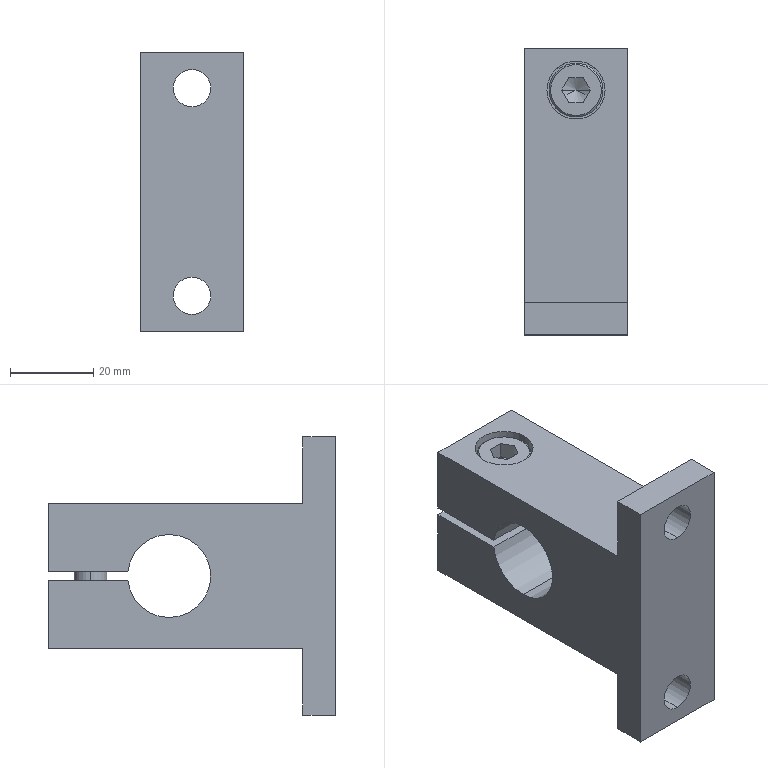Part | STEP file | 001-011-GCY02-D20-H40 | 2 solids | 52 faces | box 25 x 69 x 67 mm | volume 55893 mm3 | plane 29 | cylinder 17 | cone 6 | commonest cylinder face diameters 9 x6 20 x3 6.647 x2 8 x2 13 x2 14 x2